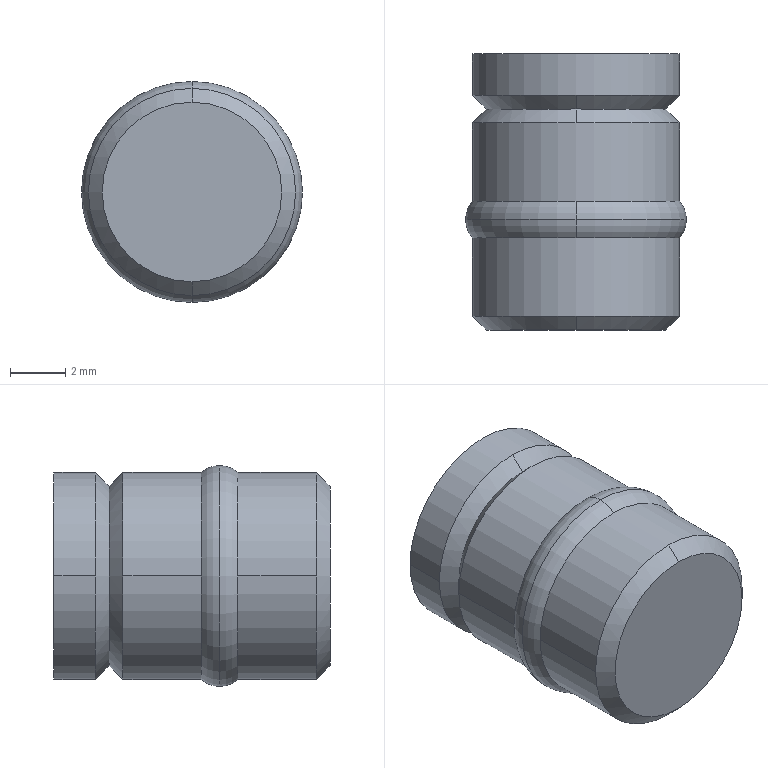Part | Creo | 1 solid | 31 faces | box 8 x 10 x 8 mm | volume 431.828 mm3 | plane 15 | cylinder 6 | cone 6 | torus 4 | commonest cylinder face diameters 7.5 x6
STEP:
#1=CARTESIAN_POINT('',(0.,0.,0.));
#2=DIRECTION('',(0.,0.,1.));
#3=DIRECTION('',(1.,0.,0.));
#4=AXIS2_PLACEMENT_3D('',#1,#2,#3);
#5=CARTESIAN_POINT('',(-58.,4.9,6.673));
#6=VERTEX_POINT('',#5);
#7=CARTESIAN_POINT('',(-59.5,4.9,6.673));
#8=VERTEX_POINT('',#7);
#9=CARTESIAN_POINT('',(-58.,4.9,6.673));
#10=DIRECTION('',(-1.,0.,0.));
#11=VECTOR('',#10,1.5);
#12=LINE('',#9,#11);
#13=EDGE_CURVE('',#6,#8,#12,.T.);
#14=ORIENTED_EDGE('',*,*,#13,.F.);
#15=CARTESIAN_POINT('',(-58.,5.9,6.673));
#16=VERTEX_POINT('',#15);
#17=CARTESIAN_POINT('',(-58.,5.9,6.673));
#18=DIRECTION('',(0.,-1.,0.));
#19=VECTOR('',#18,1.);
#20=LINE('',#17,#19);
#21=EDGE_CURVE('',#16,#6,#20,.T.);
#22=ORIENTED_EDGE('',*,*,#21,.F.);
#23=CARTESIAN_POINT('',(-59.5,5.9,6.673));
#24=VERTEX_POINT('',#23);
#25=CARTESIAN_POINT('',(-58.,5.9,6.673));
#26=DIRECTION('',(-1.,0.,0.));
#27=VECTOR('',#26,1.5);
#28=LINE('',#25,#27);
#29=EDGE_CURVE('',#16,#24,#28,.T.);
#30=ORIENTED_EDGE('',*,*,#29,.T.);
#31=CARTESIAN_POINT('',(-59.5,5.9,6.673));
#32=DIRECTION('',(0.,-1.,0.));
#33=VECTOR('',#32,1.);
#34=LINE('',#31,#33);
#35=EDGE_CURVE('',#24,#8,#34,.T.);
#36=ORIENTED_EDGE('',*,*,#35,.T.);
#37=EDGE_LOOP('',(#14,#22,#30,#36));
#38=FACE_OUTER_BOUND('',#37,.F.);
#39=CARTESIAN_POINT('',(-60.,5.4,6.673));
#40=DIRECTION('',(0.,0.,1.));
#41=DIRECTION('',(0.,1.,0.));
#42=AXIS2_PLACEMENT_3D('',#39,#40,#41);
#43=PLANE('',#42);
#44=ADVANCED_FACE('',(#38),#43,.F.);
#45=CARTESIAN_POINT('',(-59.5,4.9,5.673));
#46=VERTEX_POINT('',#45);
#47=CARTESIAN_POINT('',(-58.,4.9,5.673));
#48=VERTEX_POINT('',#47);
#49=CARTESIAN_POINT('',(-59.5,4.9,5.673));
#50=DIRECTION('',(1.,0.,0.));
#51=VECTOR('',#50,1.5);
#52=LINE('',#49,#51);
#53=EDGE_CURVE('',#46,#48,#52,.T.);
#54=ORIENTED_EDGE('',*,*,#53,.T.);
#55=CARTESIAN_POINT('',(-58.,4.9,5.673));
#56=DIRECTION('',(0.,0.,1.));
#57=VECTOR('',#56,1.);
#58=LINE('',#55,#57);
#59=EDGE_CURVE('',#48,#6,#58,.T.);
#60=ORIENTED_EDGE('',*,*,#59,.T.);
#61=ORIENTED_EDGE('',*,*,#13,.T.);
#62=CARTESIAN_POINT('',(-59.5,4.9,8.172));
#63=VERTEX_POINT('',#62);
#64=CARTESIAN_POINT('',(-59.5,4.9,8.172));
#65=DIRECTION('',(0.,0.,-1.));
#66=VECTOR('',#65,1.5);
#67=LINE('',#64,#66);
#68=EDGE_CURVE('',#63,#8,#67,.T.);
#69=ORIENTED_EDGE('',*,*,#68,.F.);
#70=CARTESIAN_POINT('',(-60.5,4.9,8.172));
#71=VERTEX_POINT('',#70);
#72=CARTESIAN_POINT('',(-60.5,4.9,8.172));
#73=DIRECTION('',(1.,0.,0.));
#74=VECTOR('',#73,1.);
#75=LINE('',#72,#74);
#76=EDGE_CURVE('',#71,#63,#75,.T.);
#77=ORIENTED_EDGE('',*,*,#76,.F.);
#78=CARTESIAN_POINT('',(-60.5,4.9,6.673));
#79=VERTEX_POINT('',#78);
#80=CARTESIAN_POINT('',(-60.5,4.9,8.172));
#81=DIRECTION('',(0.,0.,-1.));
#82=VECTOR('',#81,1.5);
#83=LINE('',#80,#82);
#84=EDGE_CURVE('',#71,#79,#83,.T.);
#85=ORIENTED_EDGE('',*,*,#84,.T.);
#86=CARTESIAN_POINT('',(-62.,4.9,6.673));
#87=VERTEX_POINT('',#86);
#88=CARTESIAN_POINT('',(-60.5,4.9,6.673));
#89=DIRECTION('',(-1.,0.,0.));
#90=VECTOR('',#89,1.5);
#91=LINE('',#88,#90);
#92=EDGE_CURVE('',#79,#87,#91,.T.);
#93=ORIENTED_EDGE('',*,*,#92,.T.);
#94=CARTESIAN_POINT('',(-62.,4.9,5.673));
#95=VERTEX_POINT('',#94);
#96=CARTESIAN_POINT('',(-62.,4.9,5.673));
#97=DIRECTION('',(0.,0.,1.));
#98=VECTOR('',#97,1.);
#99=LINE('',#96,#98);
#100=EDGE_CURVE('',#95,#87,#99,.T.);
#101=ORIENTED_EDGE('',*,*,#100,.F.);
#102=CARTESIAN_POINT('',(-60.5,4.9,5.673));
#103=VERTEX_POINT('',#102);
#104=CARTESIAN_POINT('',(-62.,4.9,5.673));
#105=DIRECTION('',(1.,0.,0.));
#106=VECTOR('',#105,1.5);
#107=LINE('',#104,#106);
#108=EDGE_CURVE('',#95,#103,#107,.T.);
#109=ORIENTED_EDGE('',*,*,#108,.T.);
#110=CARTESIAN_POINT('',(-60.5,4.9,4.173));
#111=VERTEX_POINT('',#110);
#112=CARTESIAN_POINT('',(-60.5,4.9,5.673));
#113=DIRECTION('',(0.,0.,-1.));
#114=VECTOR('',#113,1.5);
#115=LINE('',#112,#114);
#116=EDGE_CURVE('',#103,#111,#115,.T.);
#117=ORIENTED_EDGE('',*,*,#116,.T.);
#118=CARTESIAN_POINT('',(-59.5,4.9,4.173));
#119=VERTEX_POINT('',#118);
#120=CARTESIAN_POINT('',(-59.5,4.9,4.173));
#121=DIRECTION('',(-1.,0.,0.));
#122=VECTOR('',#121,1.);
#123=LINE('',#120,#122);
#124=EDGE_CURVE('',#119,#111,#123,.T.);
#125=ORIENTED_EDGE('',*,*,#124,.F.);
#126=CARTESIAN_POINT('',(-59.5,4.9,5.673));
#127=DIRECTION('',(0.,0.,-1.));
#128=VECTOR('',#127,1.5);
#129=LINE('',#126,#128);
#130=EDGE_CURVE('',#46,#119,#129,.T.);
#131=ORIENTED_EDGE('',*,*,#130,.F.);
#132=EDGE_LOOP('',(#54,#60,#61,#69,#77,#85,#93,#101,#109,#117,#125,#131));
#133=FACE_OUTER_BOUND('',#132,.F.);
#134=CARTESIAN_POINT('',(-60.,4.9,5.673));
#135=DIRECTION('',(0.,-1.,0.));
#136=DIRECTION('',(0.,0.,1.));
#137=AXIS2_PLACEMENT_3D('',#134,#135,#136);
#138=PLANE('',#137);
#139=ADVANCED_FACE('',(#133),#138,.F.);
#140=CARTESIAN_POINT('',(-59.5,5.9,5.673));
#141=VERTEX_POINT('',#140);
#142=CARTESIAN_POINT('',(-58.,5.9,5.673));
#143=VERTEX_POINT('',#142);
#144=CARTESIAN_POINT('',(-59.5,5.9,5.673));
#145=DIRECTION('',(1.,0.,0.));
#146=VECTOR('',#145,1.5);
#147=LINE('',#144,#146);
#148=EDGE_CURVE('',#141,#143,#147,.T.);
#149=ORIENTED_EDGE('',*,*,#148,.T.);
#150=CARTESIAN_POINT('',(-58.,4.9,5.673));
#151=DIRECTION('',(0.,1.,0.));
#152=VECTOR('',#151,1.);
#153=LINE('',#150,#152);
#154=EDGE_CURVE('',#48,#143,#153,.T.);
#155=ORIENTED_EDGE('',*,*,#154,.F.);
#156=ORIENTED_EDGE('',*,*,#53,.F.);
#157=CARTESIAN_POINT('',(-59.5,4.9,5.673));
#158=DIRECTION('',(0.,1.,0.));
#159=VECTOR('',#158,1.);
#160=LINE('',#157,#159);
#161=EDGE_CURVE('',#46,#141,#160,.T.);
#162=ORIENTED_EDGE('',*,*,#161,.T.);
#163=EDGE_LOOP('',(#149,#155,#156,#162));
#164=FACE_OUTER_BOUND('',#163,.F.);
#165=CARTESIAN_POINT('',(-60.,5.4,5.673));
#166=DIRECTION('',(0.,0.,-1.));
#167=DIRECTION('',(0.,-1.,0.));
#168=AXIS2_PLACEMENT_3D('',#165,#166,#167);
#169=PLANE('',#168);
#170=ADVANCED_FACE('',(#164),#169,.F.);
#171=CARTESIAN_POINT('',(-63.75,5.9,6.173));
#172=VERTEX_POINT('',#171);
#173=CARTESIAN_POINT('',(-56.25,5.9,6.173));
#174=VERTEX_POINT('',#173);
#175=CARTESIAN_POINT('',(-60.,5.9,6.173));
#176=DIRECTION('',(0.,1.,0.));
#177=DIRECTION('',(-1.,0.,0.));
#178=AXIS2_PLACEMENT_3D('',#175,#176,#177);
#179=CIRCLE('',#178,3.75);
#180=EDGE_CURVE('',#172,#174,#179,.T.);
#181=ORIENTED_EDGE('',*,*,#180,.F.);
#182=CARTESIAN_POINT('',(-60.,5.9,6.173));
#183=DIRECTION('',(0.,1.,0.));
#184=DIRECTION('',(1.,0.,0.));
#185=AXIS2_PLACEMENT_3D('',#182,#183,#184);
#186=CIRCLE('',#185,3.75);
#187=EDGE_CURVE('',#174,#172,#186,.T.);
#188=ORIENTED_EDGE('',*,*,#187,.F.);
#189=EDGE_LOOP('',(#181,#188));
#190=FACE_OUTER_BOUND('',#189,.F.);
#191=CARTESIAN_POINT('',(-60.5,5.9,5.673));
#192=VERTEX_POINT('',#191);
#193=CARTESIAN_POINT('',(-60.5,5.9,4.173));
#194=VERTEX_POINT('',#193);
#195=CARTESIAN_POINT('',(-60.5,5.9,5.673));
#196=DIRECTION('',(0.,0.,-1.));
#197=VECTOR('',#196,1.5);
#198=LINE('',#195,#197);
#199=EDGE_CURVE('',#192,#194,#198,.T.);
#200=ORIENTED_EDGE('',*,*,#199,.F.);
#201=CARTESIAN_POINT('',(-62.,5.9,5.673));
#202=VERTEX_POINT('',#201);
#203=CARTESIAN_POINT('',(-62.,5.9,5.673));
#204=DIRECTION('',(1.,0.,0.));
#205=VECTOR('',#204,1.5);
#206=LINE('',#203,#205);
#207=EDGE_CURVE('',#202,#192,#206,.T.);
#208=ORIENTED_EDGE('',*,*,#207,.F.);
#209=CARTESIAN_POINT('',(-62.,5.9,6.673));
#210=VERTEX_POINT('',#209);
#211=CARTESIAN_POINT('',(-62.,5.9,6.673));
#212=DIRECTION('',(0.,0.,-1.));
#213=VECTOR('',#212,1.);
#214=LINE('',#211,#213);
#215=EDGE_CURVE('',#210,#202,#214,.T.);
#216=ORIENTED_EDGE('',*,*,#215,.F.);
#217=CARTESIAN_POINT('',(-60.5,5.9,6.673));
#218=VERTEX_POINT('',#217);
#219=CARTESIAN_POINT('',(-60.5,5.9,6.673));
#220=DIRECTION('',(-1.,0.,0.));
#221=VECTOR('',#220,1.5);
#222=LINE('',#219,#221);
#223=EDGE_CURVE('',#218,#210,#222,.T.);
#224=ORIENTED_EDGE('',*,*,#223,.F.);
#225=CARTESIAN_POINT('',(-60.5,5.9,8.172));
#226=VERTEX_POINT('',#225);
#227=CARTESIAN_POINT('',(-60.5,5.9,8.172));
#228=DIRECTION('',(0.,0.,-1.));
#229=VECTOR('',#228,1.5);
#230=LINE('',#227,#229);
#231=EDGE_CURVE('',#226,#218,#230,.T.);
#232=ORIENTED_EDGE('',*,*,#231,.F.);
#233=CARTESIAN_POINT('',(-59.5,5.9,8.172));
#234=VERTEX_POINT('',#233);
#235=CARTESIAN_POINT('',(-59.5,5.9,8.172));
#236=DIRECTION('',(-1.,0.,0.));
#237=VECTOR('',#236,1.);
#238=LINE('',#235,#237);
#239=EDGE_CURVE('',#234,#226,#238,.T.);
#240=ORIENTED_EDGE('',*,*,#239,.F.);
#241=CARTESIAN_POINT('',(-59.5,5.9,8.172));
#242=DIRECTION('',(0.,0.,-1.));
#243=VECTOR('',#242,1.5);
#244=LINE('',#241,#243);
#245=EDGE_CURVE('',#234,#24,#244,.T.);
#246=ORIENTED_EDGE('',*,*,#245,.T.);
#247=ORIENTED_EDGE('',*,*,#29,.F.);
#248=CARTESIAN_POINT('',(-58.,5.9,6.673));
#249=DIRECTION('',(0.,0.,-1.));
#250=VECTOR('',#249,1.);
#251=LINE('',#248,#250);
#252=EDGE_CURVE('',#16,#143,#251,.T.);
#253=ORIENTED_EDGE('',*,*,#252,.T.);
#254=ORIENTED_EDGE('',*,*,#148,.F.);
#255=CARTESIAN_POINT('',(-59.5,5.9,4.173));
#256=VERTEX_POINT('',#255);
#257=CARTESIAN_POINT('',(-59.5,5.9,5.673));
#258=DIRECTION('',(0.,0.,-1.));
#259=VECTOR('',#258,1.5);
#260=LINE('',#257,#259);
#261=EDGE_CURVE('',#141,#256,#260,.T.);
#262=ORIENTED_EDGE('',*,*,#261,.T.);
#263=CARTESIAN_POINT('',(-60.5,5.9,4.173));
#264=DIRECTION('',(1.,0.,0.));
#265=VECTOR('',#264,1.);
#266=LINE('',#263,#265);
#267=EDGE_CURVE('',#194,#256,#266,.T.);
#268=ORIENTED_EDGE('',*,*,#267,.F.);
#269=EDGE_LOOP('',(#200,#208,#216,#224,#232,#240,#246,#247,#253,#254,#262,#268));
#270=FACE_BOUND('',#269,.F.);
#271=CARTESIAN_POINT('',(-60.,5.9,6.173));
#272=DIRECTION('',(0.,1.,0.));
#273=DIRECTION('',(0.,0.,1.));
#274=AXIS2_PLACEMENT_3D('',#271,#272,#273);
#275=PLANE('',#274);
#276=ADVANCED_FACE('',(#190,#270),#275,.T.);
#277=ORIENTED_EDGE('',*,*,#116,.F.);
#278=CARTESIAN_POINT('',(-60.5,5.9,5.673));
#279=DIRECTION('',(0.,-1.,0.));
#280=VECTOR('',#279,1.);
#281=LINE('',#278,#280);
#282=EDGE_CURVE('',#192,#103,#281,.T.);
#283=ORIENTED_EDGE('',*,*,#282,.F.);
#284=ORIENTED_EDGE('',*,*,#199,.T.);
#285=CARTESIAN_POINT('',(-60.5,5.9,4.173));
#286=DIRECTION('',(0.,-1.,0.));
#287=VECTOR('',#286,1.);
#288=LINE('',#285,#287);
#289=EDGE_CURVE('',#194,#111,#288,.T.);
#290=ORIENTED_EDGE('',*,*,#289,.T.);
#291=EDGE_LOOP('',(#277,#283,#284,#290));
#292=FACE_OUTER_BOUND('',#291,.F.);
#293=CARTESIAN_POINT('',(-60.5,5.4,4.173));
#294=DIRECTION('',(-1.,0.,0.));
#295=DIRECTION('',(0.,0.,1.));
#296=AXIS2_PLACEMENT_3D('',#293,#294,#295);
#297=PLANE('',#296);
#298=ADVANCED_FACE('',(#292),#297,.F.);
#299=ORIENTED_EDGE('',*,*,#108,.F.);
#300=CARTESIAN_POINT('',(-62.,5.9,5.673));
#301=DIRECTION('',(0.,-1.,0.));
#302=VECTOR('',#301,1.);
#303=LINE('',#300,#302);
#304=EDGE_CURVE('',#202,#95,#303,.T.);
#305=ORIENTED_EDGE('',*,*,#304,.F.);
#306=ORIENTED_EDGE('',*,*,#207,.T.);
#307=ORIENTED_EDGE('',*,*,#282,.T.);
#308=EDGE_LOOP('',(#299,#305,#306,#307));
#309=FACE_OUTER_BOUND('',#308,.F.);
#310=CARTESIAN_POINT('',(-60.,5.4,5.673));
#311=DIRECTION('',(0.,0.,-1.));
#312=DIRECTION('',(0.,-1.,0.));
#313=AXIS2_PLACEMENT_3D('',#310,#311,#312);
#314=PLANE('',#313);
#315=ADVANCED_FACE('',(#309),#314,.F.);
#316=ORIENTED_EDGE('',*,*,#100,.T.);
#317=CARTESIAN_POINT('',(-62.,4.9,6.673));
#318=DIRECTION('',(0.,1.,0.));
#319=VECTOR('',#318,1.);
#320=LINE('',#317,#319);
#321=EDGE_CURVE('',#87,#210,#320,.T.);
#322=ORIENTED_EDGE('',*,*,#321,.T.);
#323=ORIENTED_EDGE('',*,*,#215,.T.);
#324=ORIENTED_EDGE('',*,*,#304,.T.);
#325=EDGE_LOOP('',(#316,#322,#323,#324));
#326=FACE_OUTER_BOUND('',#325,.F.);
#327=CARTESIAN_POINT('',(-62.,5.4,5.673));
#328=DIRECTION('',(-1.,0.,0.));
#329=DIRECTION('',(0.,0.,1.));
#330=AXIS2_PLACEMENT_3D('',#327,#328,#329);
#331=PLANE('',#330);
#332=ADVANCED_FACE('',(#326),#331,.F.);
#333=ORIENTED_EDGE('',*,*,#223,.T.);
#334=ORIENTED_EDGE('',*,*,#321,.F.);
#335=ORIENTED_EDGE('',*,*,#92,.F.);
#336=CARTESIAN_POINT('',(-60.5,4.9,6.673));
#337=DIRECTION('',(0.,1.,0.));
#338=VECTOR('',#337,1.);
#339=LINE('',#336,#338);
#340=EDGE_CURVE('',#79,#218,#339,.T.);
#341=ORIENTED_EDGE('',*,*,#340,.T.);
#342=EDGE_LOOP('',(#333,#334,#335,#341));
#343=FACE_OUTER_BOUND('',#342,.F.);
#344=CARTESIAN_POINT('',(-60.,5.4,6.673));
#345=DIRECTION('',(0.,0.,1.));
#346=DIRECTION('',(0.,1.,0.));
#347=AXIS2_PLACEMENT_3D('',#344,#345,#346);
#348=PLANE('',#347);
#349=ADVANCED_FACE('',(#343),#348,.F.);
#350=ORIENTED_EDGE('',*,*,#231,.T.);
#351=ORIENTED_EDGE('',*,*,#340,.F.);
#352=ORIENTED_EDGE('',*,*,#84,.F.);
#353=CARTESIAN_POINT('',(-60.5,4.9,8.172));
#354=DIRECTION('',(0.,1.,0.));
#355=VECTOR('',#354,1.);
#356=LINE('',#353,#355);
#357=EDGE_CURVE('',#71,#226,#356,.T.);
#358=ORIENTED_EDGE('',*,*,#357,.T.);
#359=EDGE_LOOP('',(#350,#351,#352,#358));
#360=FACE_OUTER_BOUND('',#359,.F.);
#361=CARTESIAN_POINT('',(-60.5,5.4,4.173));
#362=DIRECTION('',(-1.,0.,0.));
#363=DIRECTION('',(0.,0.,1.));
#364=AXIS2_PLACEMENT_3D('',#361,#362,#363);
#365=PLANE('',#364);
#366=ADVANCED_FACE('',(#360),#365,.F.);
#367=CARTESIAN_POINT('',(-59.5,5.9,8.172));
#368=DIRECTION('',(0.,-1.,0.));
#369=VECTOR('',#368,1.);
#370=LINE('',#367,#369);
#371=EDGE_CURVE('',#234,#63,#370,.T.);
#372=ORIENTED_EDGE('',*,*,#371,.F.);
#373=ORIENTED_EDGE('',*,*,#239,.T.);
#374=ORIENTED_EDGE('',*,*,#357,.F.);
#375=ORIENTED_EDGE('',*,*,#76,.T.);
#376=EDGE_LOOP('',(#372,#373,#374,#375));
#377=FACE_OUTER_BOUND('',#376,.F.);
#378=CARTESIAN_POINT('',(-60.,5.4,8.172));
#379=DIRECTION('',(0.,0.,1.));
#380=DIRECTION('',(0.,1.,0.));
#381=AXIS2_PLACEMENT_3D('',#378,#379,#380);
#382=PLANE('',#381);
#383=ADVANCED_FACE('',(#377),#382,.F.);
#384=ORIENTED_EDGE('',*,*,#68,.T.);
#385=ORIENTED_EDGE('',*,*,#35,.F.);
#386=ORIENTED_EDGE('',*,*,#245,.F.);
#387=ORIENTED_EDGE('',*,*,#371,.T.);
#388=EDGE_LOOP('',(#384,#385,#386,#387));
#389=FACE_OUTER_BOUND('',#388,.F.);
#390=CARTESIAN_POINT('',(-59.5,5.4,4.173));
#391=DIRECTION('',(1.,0.,0.));
#392=DIRECTION('',(0.,0.,-1.));
#393=AXIS2_PLACEMENT_3D('',#390,#391,#392);
#394=PLANE('',#393);
#395=ADVANCED_FACE('',(#389),#394,.F.);
#396=ORIENTED_EDGE('',*,*,#267,.T.);
#397=CARTESIAN_POINT('',(-59.5,4.9,4.173));
#398=DIRECTION('',(0.,1.,0.));
#399=VECTOR('',#398,1.);
#400=LINE('',#397,#399);
#401=EDGE_CURVE('',#119,#256,#400,.T.);
#402=ORIENTED_EDGE('',*,*,#401,.F.);
#403=ORIENTED_EDGE('',*,*,#124,.T.);
#404=ORIENTED_EDGE('',*,*,#289,.F.);
#405=EDGE_LOOP('',(#396,#402,#403,#404));
#406=FACE_OUTER_BOUND('',#405,.F.);
#407=CARTESIAN_POINT('',(-60.,5.4,4.173));
#408=DIRECTION('',(0.,0.,-1.));
#409=DIRECTION('',(0.,-1.,0.));
#410=AXIS2_PLACEMENT_3D('',#407,#408,#409);
#411=PLANE('',#410);
#412=ADVANCED_FACE('',(#406),#411,.F.);
#413=ORIENTED_EDGE('',*,*,#261,.F.);
#414=ORIENTED_EDGE('',*,*,#161,.F.);
#415=ORIENTED_EDGE('',*,*,#130,.T.);
#416=ORIENTED_EDGE('',*,*,#401,.T.);
#417=EDGE_LOOP('',(#413,#414,#415,#416));
#418=FACE_OUTER_BOUND('',#417,.F.);
#419=CARTESIAN_POINT('',(-59.5,5.4,4.173));
#420=DIRECTION('',(1.,0.,0.));
#421=DIRECTION('',(0.,0.,-1.));
#422=AXIS2_PLACEMENT_3D('',#419,#420,#421);
#423=PLANE('',#422);
#424=ADVANCED_FACE('',(#418),#423,.F.);
#425=ORIENTED_EDGE('',*,*,#252,.F.);
#426=ORIENTED_EDGE('',*,*,#21,.T.);
#427=ORIENTED_EDGE('',*,*,#59,.F.);
#428=ORIENTED_EDGE('',*,*,#154,.T.);
#429=EDGE_LOOP('',(#425,#426,#427,#428));
#430=FACE_OUTER_BOUND('',#429,.F.);
#431=CARTESIAN_POINT('',(-58.,5.4,5.673));
#432=DIRECTION('',(1.,0.,0.));
#433=DIRECTION('',(0.,0.,-1.));
#434=AXIS2_PLACEMENT_3D('',#431,#432,#433);
#435=PLANE('',#434);
#436=ADVANCED_FACE('',(#430),#435,.F.);
#437=CARTESIAN_POINT('',(-60.,4.4,9.922));
#438=VERTEX_POINT('',#437);
#439=CARTESIAN_POINT('',(-63.75,4.4,6.173));
#440=VERTEX_POINT('',#439);
#441=CARTESIAN_POINT('',(-60.,4.4,6.173));
#442=DIRECTION('',(0.,-1.,0.));
#443=DIRECTION('',(0.,0.,1.));
#444=AXIS2_PLACEMENT_3D('',#441,#442,#443);
#445=CIRCLE('',#444,3.75);
#446=EDGE_CURVE('',#438,#440,#445,.T.);
#447=ORIENTED_EDGE('',*,*,#446,.T.);
#448=CARTESIAN_POINT('',(-63.75,5.9,6.173));
#449=DIRECTION('',(0.,-1.,0.));
#450=VECTOR('',#449,1.5);
#451=LINE('',#448,#450);
#452=EDGE_CURVE('',#172,#440,#451,.T.);
#453=ORIENTED_EDGE('',*,*,#452,.F.);
#454=ORIENTED_EDGE('',*,*,#180,.T.);
#455=CARTESIAN_POINT('',(-56.25,4.4,6.173));
#456=VERTEX_POINT('',#455);
#457=CARTESIAN_POINT('',(-56.25,5.9,6.173));
#458=DIRECTION('',(0.,-1.,0.));
#459=VECTOR('',#458,1.5);
#460=LINE('',#457,#459);
#461=EDGE_CURVE('',#174,#456,#460,.T.);
#462=ORIENTED_EDGE('',*,*,#461,.T.);
#463=CARTESIAN_POINT('',(-60.,4.4,6.173));
#464=DIRECTION('',(0.,-1.,0.));
#465=DIRECTION('',(1.,0.,0.));
#466=AXIS2_PLACEMENT_3D('',#463,#464,#465);
#467=CIRCLE('',#466,3.75);
#468=EDGE_CURVE('',#456,#438,#467,.T.);
#469=ORIENTED_EDGE('',*,*,#468,.T.);
#470=EDGE_LOOP('',(#447,#453,#454,#462,#469));
#471=FACE_OUTER_BOUND('',#470,.F.);
#472=CARTESIAN_POINT('',(-60.,5.9,6.173));
#473=DIRECTION('',(0.,-1.,0.));
#474=DIRECTION('',(-1.,0.,0.));
#475=AXIS2_PLACEMENT_3D('',#472,#473,#474);
#476=CYLINDRICAL_SURFACE('',#475,3.75);
#477=ADVANCED_FACE('',(#471),#476,.T.);
#478=CARTESIAN_POINT('',(-60.,3.9,2.922));
#479=VERTEX_POINT('',#478);
#480=CARTESIAN_POINT('',(-60.,3.9,9.422));
#481=VERTEX_POINT('',#480);
#482=CARTESIAN_POINT('',(-60.,3.9,6.173));
#483=DIRECTION('',(0.,1.,0.));
#484=DIRECTION('',(0.,0.,-1.));
#485=AXIS2_PLACEMENT_3D('',#482,#483,#484);
#486=CIRCLE('',#485,3.25);
#487=EDGE_CURVE('',#479,#481,#486,.T.);
#488=ORIENTED_EDGE('',*,*,#487,.F.);
#489=CARTESIAN_POINT('',(-60.,4.4,2.422));
#490=VERTEX_POINT('',#489);
#491=CARTESIAN_POINT('',(-60.,3.9,2.922));
#492=DIRECTION('',(0.,0.7071,-0.7071));
#493=VECTOR('',#492,0.7071);
#494=LINE('',#491,#493);
#495=EDGE_CURVE('',#479,#490,#494,.T.);
#496=ORIENTED_EDGE('',*,*,#495,.T.);
#497=CARTESIAN_POINT('',(-60.,4.4,6.173));
#498=DIRECTION('',(0.,-1.,0.));
#499=DIRECTION('',(-1.,0.,0.));
#500=AXIS2_PLACEMENT_3D('',#497,#498,#499);
#501=CIRCLE('',#500,3.75);
#502=EDGE_CURVE('',#440,#490,#501,.T.);
#503=ORIENTED_EDGE('',*,*,#502,.F.);
#504=ORIENTED_EDGE('',*,*,#446,.F.);
#505=CARTESIAN_POINT('',(-60.,3.9,9.422));
#506=DIRECTION('',(0.,0.7071,0.7071));
#507=VECTOR('',#506,0.7071);
#508=LINE('',#505,#507);
#509=EDGE_CURVE('',#481,#438,#508,.T.);
#510=ORIENTED_EDGE('',*,*,#509,.F.);
#511=EDGE_LOOP('',(#488,#496,#503,#504,#510));
#512=FACE_OUTER_BOUND('',#511,.F.);
#513=CARTESIAN_POINT('',(-60.,4.15,6.173));
#514=DIRECTION('',(0.,1.,0.));
#515=DIRECTION('',(0.,0.,1.));
#516=AXIS2_PLACEMENT_3D('',#513,#514,#515);
#517=CONICAL_SURFACE('',#516,3.5,45.);
#518=ADVANCED_FACE('',(#512),#517,.T.);
#519=ORIENTED_EDGE('',*,*,#487,.T.);
#520=CARTESIAN_POINT('',(-60.,3.4,9.922));
#521=VERTEX_POINT('',#520);
#522=CARTESIAN_POINT('',(-60.,3.9,9.422));
#523=DIRECTION('',(0.,-0.7071,0.7071));
#524=VECTOR('',#523,0.7071);
#525=LINE('',#522,#524);
#526=EDGE_CURVE('',#481,#521,#525,.T.);
#527=ORIENTED_EDGE('',*,*,#526,.T.);
#528=CARTESIAN_POINT('',(-63.75,3.4,6.173));
#529=VERTEX_POINT('',#528);
#530=CARTESIAN_POINT('',(-60.,3.4,6.173));
#531=DIRECTION('',(0.,1.,0.));
#532=DIRECTION('',(-1.,0.,0.));
#533=AXIS2_PLACEMENT_3D('',#530,#531,#532);
#534=CIRCLE('',#533,3.75);
#535=EDGE_CURVE('',#529,#521,#534,.T.);
#536=ORIENTED_EDGE('',*,*,#535,.F.);
#537=CARTESIAN_POINT('',(-60.,3.4,2.422));
#538=VERTEX_POINT('',#537);
#539=CARTESIAN_POINT('',(-60.,3.4,6.173));
#540=DIRECTION('',(0.,1.,0.));
#541=DIRECTION('',(0.,0.,-1.));
#542=AXIS2_PLACEMENT_3D('',#539,#540,#541);
#543=CIRCLE('',#542,3.75);
#544=EDGE_CURVE('',#538,#529,#543,.T.);
#545=ORIENTED_EDGE('',*,*,#544,.F.);
#546=CARTESIAN_POINT('',(-60.,3.9,2.922));
#547=DIRECTION('',(0.,-0.7071,-0.7071));
#548=VECTOR('',#547,0.7071);
#549=LINE('',#546,#548);
#550=EDGE_CURVE('',#479,#538,#549,.T.);
#551=ORIENTED_EDGE('',*,*,#550,.F.);
#552=EDGE_LOOP('',(#519,#527,#536,#545,#551));
#553=FACE_OUTER_BOUND('',#552,.F.);
#554=CARTESIAN_POINT('',(-60.,3.65,6.173));
#555=DIRECTION('',(0.,-1.,0.));
#556=DIRECTION('',(0.,0.,-1.));
#557=AXIS2_PLACEMENT_3D('',#554,#555,#556);
#558=CONICAL_SURFACE('',#557,3.5,45.);
#559=ADVANCED_FACE('',(#553),#558,.T.);
#560=CARTESIAN_POINT('',(-60.,3.9,6.173));
#561=DIRECTION('',(0.,1.,0.));
#562=DIRECTION('',(0.,0.,1.));
#563=AXIS2_PLACEMENT_3D('',#560,#561,#562);
#564=CIRCLE('',#563,3.25);
#565=EDGE_CURVE('',#481,#479,#564,.T.);
#566=ORIENTED_EDGE('',*,*,#565,.T.);
#567=ORIENTED_EDGE('',*,*,#550,.T.);
#568=CARTESIAN_POINT('',(-56.25,3.4,6.173));
#569=VERTEX_POINT('',#568);
#570=CARTESIAN_POINT('',(-60.,3.4,6.173));
#571=DIRECTION('',(0.,1.,0.));
#572=DIRECTION('',(1.,0.,0.));
#573=AXIS2_PLACEMENT_3D('',#570,#571,#572);
#574=CIRCLE('',#573,3.75);
#575=EDGE_CURVE('',#569,#538,#574,.T.);
#576=ORIENTED_EDGE('',*,*,#575,.F.);
#577=CARTESIAN_POINT('',(-60.,3.4,6.173));
#578=DIRECTION('',(0.,1.,0.));
#579=DIRECTION('',(0.,0.,1.));
#580=AXIS2_PLACEMENT_3D('',#577,#578,#579);
#581=CIRCLE('',#580,3.75);
#582=EDGE_CURVE('',#521,#569,#581,.T.);
#583=ORIENTED_EDGE('',*,*,#582,.F.);
#584=ORIENTED_EDGE('',*,*,#526,.F.);
#585=EDGE_LOOP('',(#566,#567,#576,#583,#584));
#586=FACE_OUTER_BOUND('',#585,.F.);
#587=CARTESIAN_POINT('',(-60.,3.65,6.173));
#588=DIRECTION('',(0.,-1.,0.));
#589=DIRECTION('',(0.,0.,-1.));
#590=AXIS2_PLACEMENT_3D('',#587,#588,#589);
#591=CONICAL_SURFACE('',#590,3.5,45.);
#592=ADVANCED_FACE('',(#586),#591,.T.);
#593=ORIENTED_EDGE('',*,*,#565,.F.);
#594=ORIENTED_EDGE('',*,*,#509,.T.);
#595=ORIENTED_EDGE('',*,*,#468,.F.);
#596=CARTESIAN_POINT('',(-60.,4.4,6.173));
#597=DIRECTION('',(0.,-1.,0.));
#598=DIRECTION('',(0.,0.,-1.));
#599=AXIS2_PLACEMENT_3D('',#596,#597,#598);
#600=CIRCLE('',#599,3.75);
#601=EDGE_CURVE('',#490,#456,#600,.T.);
#602=ORIENTED_EDGE('',*,*,#601,.F.);
#603=ORIENTED_EDGE('',*,*,#495,.F.);
#604=EDGE_LOOP('',(#593,#594,#595,#602,#603));
#605=FACE_OUTER_BOUND('',#604,.F.);
#606=CARTESIAN_POINT('',(-60.,4.15,6.173));
#607=DIRECTION('',(0.,1.,0.));
#608=DIRECTION('',(0.,0.,1.));
#609=AXIS2_PLACEMENT_3D('',#606,#607,#608);
#610=CONICAL_SURFACE('',#609,3.5,45.);
#611=ADVANCED_FACE('',(#605),#610,.T.);
#612=ORIENTED_EDGE('',*,*,#502,.T.);
#613=ORIENTED_EDGE('',*,*,#601,.T.);
#614=ORIENTED_EDGE('',*,*,#461,.F.);
#615=ORIENTED_EDGE('',*,*,#187,.T.);
#616=ORIENTED_EDGE('',*,*,#452,.T.);
#617=EDGE_LOOP('',(#612,#613,#614,#615,#616));
#618=FACE_OUTER_BOUND('',#617,.F.);
#619=CARTESIAN_POINT('',(-60.,5.9,6.173));
#620=DIRECTION('',(0.,-1.,0.));
#621=DIRECTION('',(-1.,0.,0.));
#622=AXIS2_PLACEMENT_3D('',#619,#620,#621);
#623=CYLINDRICAL_SURFACE('',#622,3.75);
#624=ADVANCED_FACE('',(#618),#623,.T.);
#625=CARTESIAN_POINT('',(-63.75,0.5614,6.173));
#626=VERTEX_POINT('',#625);
#627=CARTESIAN_POINT('',(-60.,0.5614,2.422));
#628=VERTEX_POINT('',#627);
#629=CARTESIAN_POINT('',(-60.,0.5614,6.173));
#630=DIRECTION('',(0.,-1.,0.));
#631=DIRECTION('',(-1.,0.,0.));
#632=AXIS2_PLACEMENT_3D('',#629,#630,#631);
#633=CIRCLE('',#632,3.75);
#634=EDGE_CURVE('',#626,#628,#633,.T.);
#635=ORIENTED_EDGE('',*,*,#634,.T.);
#636=CARTESIAN_POINT('',(-56.25,0.5614,6.173));
#637=VERTEX_POINT('',#636);
#638=CARTESIAN_POINT('',(-60.,0.5614,6.173));
#639=DIRECTION('',(0.,-1.,0.));
#640=DIRECTION('',(0.,0.,-1.));
#641=AXIS2_PLACEMENT_3D('',#638,#639,#640);
#642=CIRCLE('',#641,3.75);
#643=EDGE_CURVE('',#628,#637,#642,.T.);
#644=ORIENTED_EDGE('',*,*,#643,.T.);
#645=CARTESIAN_POINT('',(-56.25,3.4,6.173));
#646=DIRECTION('',(0.,-1.,0.));
#647=VECTOR('',#646,2.839);
#648=LINE('',#645,#647);
#649=EDGE_CURVE('',#569,#637,#648,.T.);
#650=ORIENTED_EDGE('',*,*,#649,.F.);
#651=ORIENTED_EDGE('',*,*,#575,.T.);
#652=ORIENTED_EDGE('',*,*,#544,.T.);
#653=CARTESIAN_POINT('',(-63.75,3.4,6.173));
#654=DIRECTION('',(0.,-1.,0.));
#655=VECTOR('',#654,2.839);
#656=LINE('',#653,#655);
#657=EDGE_CURVE('',#529,#626,#656,.T.);
#658=ORIENTED_EDGE('',*,*,#657,.T.);
#659=EDGE_LOOP('',(#635,#644,#650,#651,#652,#658));
#660=FACE_OUTER_BOUND('',#659,.F.);
#661=CARTESIAN_POINT('',(-60.,3.9,6.173));
#662=DIRECTION('',(0.,-1.,0.));
#663=DIRECTION('',(-1.,0.,0.));
#664=AXIS2_PLACEMENT_3D('',#661,#662,#663);
#665=CYLINDRICAL_SURFACE('',#664,3.75);
#666=ADVANCED_FACE('',(#660),#665,.T.);
#667=CARTESIAN_POINT('',(-60.,0.5614,9.922));
#668=VERTEX_POINT('',#667);
#669=CARTESIAN_POINT('',(-60.,0.5614,6.173));
#670=DIRECTION('',(0.,-1.,0.));
#671=DIRECTION('',(0.,0.,1.));
#672=AXIS2_PLACEMENT_3D('',#669,#670,#671);
#673=CIRCLE('',#672,3.75);
#674=EDGE_CURVE('',#668,#626,#673,.T.);
#675=ORIENTED_EDGE('',*,*,#674,.F.);
#676=CARTESIAN_POINT('',(-60.,-0.1,10.172));
#677=VERTEX_POINT('',#676);
#678=CARTESIAN_POINT('',(-60.,-0.1,9.172));
#679=DIRECTION('',(-1.,0.,0.));
#680=DIRECTION('',(0.,0.,1.));
#681=AXIS2_PLACEMENT_3D('',#678,#679,#680);
#682=CIRCLE('',#681,1.);
#683=EDGE_CURVE('',#677,#668,#682,.T.);
#684=ORIENTED_EDGE('',*,*,#683,.F.);
#685=CARTESIAN_POINT('',(-60.,-0.1,2.172));
#686=VERTEX_POINT('',#685);
#687=CARTESIAN_POINT('',(-60.,-0.1,6.173));
#688=DIRECTION('',(0.,1.,0.));
#689=DIRECTION('',(0.,0.,-1.));
#690=AXIS2_PLACEMENT_3D('',#687,#688,#689);
#691=CIRCLE('',#690,4.);
#692=EDGE_CURVE('',#686,#677,#691,.T.);
#693=ORIENTED_EDGE('',*,*,#692,.F.);
#694=CARTESIAN_POINT('',(-60.,-0.1,3.172));
#695=DIRECTION('',(1.,0.,0.));
#696=DIRECTION('',(0.,0.,-1.));
#697=AXIS2_PLACEMENT_3D('',#694,#695,#696);
#698=CIRCLE('',#697,1.);
#699=EDGE_CURVE('',#686,#628,#698,.T.);
#700=ORIENTED_EDGE('',*,*,#699,.T.);
#701=ORIENTED_EDGE('',*,*,#634,.F.);
#702=EDGE_LOOP('',(#675,#684,#693,#700,#701));
#703=FACE_OUTER_BOUND('',#702,.F.);
#704=CARTESIAN_POINT('',(-60.,-0.1,6.173));
#705=DIRECTION('',(0.,1.,0.));
#706=DIRECTION('',(0.,0.,1.));
#707=AXIS2_PLACEMENT_3D('',#704,#705,#706);
#708=TOROIDAL_SURFACE('',#707,3.,1.);
#709=ADVANCED_FACE('',(#703),#708,.T.);
#710=ORIENTED_EDGE('',*,*,#674,.T.);
#711=ORIENTED_EDGE('',*,*,#657,.F.);
#712=ORIENTED_EDGE('',*,*,#535,.T.);
#713=ORIENTED_EDGE('',*,*,#582,.T.);
#714=ORIENTED_EDGE('',*,*,#649,.T.);
#715=CARTESIAN_POINT('',(-60.,0.5614,6.173));
#716=DIRECTION('',(0.,-1.,0.));
#717=DIRECTION('',(1.,0.,0.));
#718=AXIS2_PLACEMENT_3D('',#715,#716,#717);
#719=CIRCLE('',#718,3.75);
#720=EDGE_CURVE('',#637,#668,#719,.T.);
#721=ORIENTED_EDGE('',*,*,#720,.T.);
#722=EDGE_LOOP('',(#710,#711,#712,#713,#714,#721));
#723=FACE_OUTER_BOUND('',#722,.F.);
#724=CARTESIAN_POINT('',(-60.,3.9,6.173));
#725=DIRECTION('',(0.,-1.,0.));
#726=DIRECTION('',(-1.,0.,0.));
#727=AXIS2_PLACEMENT_3D('',#724,#725,#726);
#728=CYLINDRICAL_SURFACE('',#727,3.75);
#729=ADVANCED_FACE('',(#723),#728,.T.);
#730=ORIENTED_EDGE('',*,*,#643,.F.);
#731=ORIENTED_EDGE('',*,*,#699,.F.);
#732=CARTESIAN_POINT('',(-60.,-0.1,6.173));
#733=DIRECTION('',(0.,1.,0.));
#734=DIRECTION('',(0.,0.,1.));
#735=AXIS2_PLACEMENT_3D('',#732,#733,#734);
#736=CIRCLE('',#735,4.);
#737=EDGE_CURVE('',#677,#686,#736,.T.);
#738=ORIENTED_EDGE('',*,*,#737,.F.);
#739=ORIENTED_EDGE('',*,*,#683,.T.);
#740=ORIENTED_EDGE('',*,*,#720,.F.);
#741=EDGE_LOOP('',(#730,#731,#738,#739,#740));
#742=FACE_OUTER_BOUND('',#741,.F.);
#743=CARTESIAN_POINT('',(-60.,-0.1,6.173));
#744=DIRECTION('',(0.,1.,0.));
#745=DIRECTION('',(0.,0.,1.));
#746=AXIS2_PLACEMENT_3D('',#743,#744,#745);
#747=TOROIDAL_SURFACE('',#746,3.,1.);
#748=ADVANCED_FACE('',(#742),#747,.T.);
#749=CARTESIAN_POINT('',(-60.,-0.7614,9.922));
#750=VERTEX_POINT('',#749);
#751=CARTESIAN_POINT('',(-56.25,-0.7614,6.173));
#752=VERTEX_POINT('',#751);
#753=CARTESIAN_POINT('',(-60.,-0.7614,6.173));
#754=DIRECTION('',(0.,1.,0.));
#755=DIRECTION('',(0.,0.,1.));
#756=AXIS2_PLACEMENT_3D('',#753,#754,#755);
#757=CIRCLE('',#756,3.75);
#758=EDGE_CURVE('',#750,#752,#757,.T.);
#759=ORIENTED_EDGE('',*,*,#758,.F.);
#760=CARTESIAN_POINT('',(-60.,-0.1,9.172));
#761=DIRECTION('',(-1.,0.,0.));
#762=DIRECTION('',(0.,-0.6614,0.75));
#763=AXIS2_PLACEMENT_3D('',#760,#761,#762);
#764=CIRCLE('',#763,1.);
#765=EDGE_CURVE('',#750,#677,#764,.T.);
#766=ORIENTED_EDGE('',*,*,#765,.T.);
#767=ORIENTED_EDGE('',*,*,#737,.T.);
#768=CARTESIAN_POINT('',(-60.,-0.7614,2.422));
#769=VERTEX_POINT('',#768);
#770=CARTESIAN_POINT('',(-60.,-0.1,3.172));
#771=DIRECTION('',(1.,0.,0.));
#772=DIRECTION('',(0.,-0.6614,-0.75));
#773=AXIS2_PLACEMENT_3D('',#770,#771,#772);
#774=CIRCLE('',#773,1.);
#775=EDGE_CURVE('',#769,#686,#774,.T.);
#776=ORIENTED_EDGE('',*,*,#775,.F.);
#777=CARTESIAN_POINT('',(-60.,-0.7614,6.173));
#778=DIRECTION('',(0.,1.,0.));
#779=DIRECTION('',(1.,0.,0.));
#780=AXIS2_PLACEMENT_3D('',#777,#778,#779);
#781=CIRCLE('',#780,3.75);
#782=EDGE_CURVE('',#752,#769,#781,.T.);
#783=ORIENTED_EDGE('',*,*,#782,.F.);
#784=EDGE_LOOP('',(#759,#766,#767,#776,#783));
#785=FACE_OUTER_BOUND('',#784,.F.);
#786=CARTESIAN_POINT('',(-60.,-0.1,6.173));
#787=DIRECTION('',(0.,1.,0.));
#788=DIRECTION('',(0.,0.,1.));
#789=AXIS2_PLACEMENT_3D('',#786,#787,#788);
#790=TOROIDAL_SURFACE('',#789,3.,1.);
#791=ADVANCED_FACE('',(#785),#790,.T.);
#792=CARTESIAN_POINT('',(-63.75,-0.7614,6.173));
#793=VERTEX_POINT('',#792);
#794=CARTESIAN_POINT('',(-60.,-0.7614,6.173));
#795=DIRECTION('',(0.,1.,0.));
#796=DIRECTION('',(-1.,0.,0.));
#797=AXIS2_PLACEMENT_3D('',#794,#795,#796);
#798=CIRCLE('',#797,3.75);
#799=EDGE_CURVE('',#793,#750,#798,.T.);
#800=ORIENTED_EDGE('',*,*,#799,.T.);
#801=ORIENTED_EDGE('',*,*,#758,.T.);
#802=CARTESIAN_POINT('',(-56.25,-3.6,6.173));
#803=VERTEX_POINT('',#802);
#804=CARTESIAN_POINT('',(-56.25,-0.7614,6.173));
#805=DIRECTION('',(0.,-1.,0.));
#806=VECTOR('',#805,2.839);
#807=LINE('',#804,#806);
#808=EDGE_CURVE('',#752,#803,#807,.T.);
#809=ORIENTED_EDGE('',*,*,#808,.T.);
#810=CARTESIAN_POINT('',(-60.,-3.6,9.922));
#811=VERTEX_POINT('',#810);
#812=CARTESIAN_POINT('',(-60.,-3.6,6.173));
#813=DIRECTION('',(0.,-1.,0.));
#814=DIRECTION('',(1.,0.,0.));
#815=AXIS2_PLACEMENT_3D('',#812,#813,#814);
#816=CIRCLE('',#815,3.75);
#817=EDGE_CURVE('',#803,#811,#816,.T.);
#818=ORIENTED_EDGE('',*,*,#817,.T.);
#819=CARTESIAN_POINT('',(-63.75,-3.6,6.173));
#820=VERTEX_POINT('',#819);
#821=CARTESIAN_POINT('',(-60.,-3.6,6.173));
#822=DIRECTION('',(0.,-1.,0.));
#823=DIRECTION('',(0.,0.,1.));
#824=AXIS2_PLACEMENT_3D('',#821,#822,#823);
#825=CIRCLE('',#824,3.75);
#826=EDGE_CURVE('',#811,#820,#825,.T.);
#827=ORIENTED_EDGE('',*,*,#826,.T.);
#828=CARTESIAN_POINT('',(-63.75,-0.7614,6.173));
#829=DIRECTION('',(0.,-1.,0.));
#830=VECTOR('',#829,2.839);
#831=LINE('',#828,#830);
#832=EDGE_CURVE('',#793,#820,#831,.T.);
#833=ORIENTED_EDGE('',*,*,#832,.F.);
#834=EDGE_LOOP('',(#800,#801,#809,#818,#827,#833));
#835=FACE_OUTER_BOUND('',#834,.F.);
#836=CARTESIAN_POINT('',(-60.,3.9,6.173));
#837=DIRECTION('',(0.,-1.,0.));
#838=DIRECTION('',(-1.,0.,0.));
#839=AXIS2_PLACEMENT_3D('',#836,#837,#838);
#840=CYLINDRICAL_SURFACE('',#839,3.75);
#841=ADVANCED_FACE('',(#835),#840,.T.);
#842=CARTESIAN_POINT('',(-60.,-0.7614,6.173));
#843=DIRECTION('',(0.,1.,0.));
#844=DIRECTION('',(0.,0.,-1.));
#845=AXIS2_PLACEMENT_3D('',#842,#843,#844);
#846=CIRCLE('',#845,3.75);
#847=EDGE_CURVE('',#769,#793,#846,.T.);
#848=ORIENTED_EDGE('',*,*,#847,.F.);
#849=ORIENTED_EDGE('',*,*,#775,.T.);
#850=ORIENTED_EDGE('',*,*,#692,.T.);
#851=ORIENTED_EDGE('',*,*,#765,.F.);
#852=ORIENTED_EDGE('',*,*,#799,.F.);
#853=EDGE_LOOP('',(#848,#849,#850,#851,#852));
#854=FACE_OUTER_BOUND('',#853,.F.);
#855=CARTESIAN_POINT('',(-60.,-0.1,6.173));
#856=DIRECTION('',(0.,1.,0.));
#857=DIRECTION('',(0.,0.,1.));
#858=AXIS2_PLACEMENT_3D('',#855,#856,#857);
#859=TOROIDAL_SURFACE('',#858,3.,1.);
#860=ADVANCED_FACE('',(#854),#859,.T.);
#861=ORIENTED_EDGE('',*,*,#847,.T.);
#862=ORIENTED_EDGE('',*,*,#832,.T.);
#863=CARTESIAN_POINT('',(-60.,-3.6,2.422));
#864=VERTEX_POINT('',#863);
#865=CARTESIAN_POINT('',(-60.,-3.6,6.173));
#866=DIRECTION('',(0.,-1.,0.));
#867=DIRECTION('',(-1.,0.,0.));
#868=AXIS2_PLACEMENT_3D('',#865,#866,#867);
#869=CIRCLE('',#868,3.75);
#870=EDGE_CURVE('',#820,#864,#869,.T.);
#871=ORIENTED_EDGE('',*,*,#870,.T.);
#872=CARTESIAN_POINT('',(-60.,-3.6,6.173));
#873=DIRECTION('',(0.,-1.,0.));
#874=DIRECTION('',(0.,0.,-1.));
#875=AXIS2_PLACEMENT_3D('',#872,#873,#874);
#876=CIRCLE('',#875,3.75);
#877=EDGE_CURVE('',#864,#803,#876,.T.);
#878=ORIENTED_EDGE('',*,*,#877,.T.);
#879=ORIENTED_EDGE('',*,*,#808,.F.);
#880=ORIENTED_EDGE('',*,*,#782,.T.);
#881=EDGE_LOOP('',(#861,#862,#871,#878,#879,#880));
#882=FACE_OUTER_BOUND('',#881,.F.);
#883=CARTESIAN_POINT('',(-60.,3.9,6.173));
#884=DIRECTION('',(0.,-1.,0.));
#885=DIRECTION('',(-1.,0.,0.));
#886=AXIS2_PLACEMENT_3D('',#883,#884,#885);
#887=CYLINDRICAL_SURFACE('',#886,3.75);
#888=ADVANCED_FACE('',(#882),#887,.T.);
#889=CARTESIAN_POINT('',(-60.,-4.1,9.422));
#890=VERTEX_POINT('',#889);
#891=CARTESIAN_POINT('',(-60.,-4.1,2.922));
#892=VERTEX_POINT('',#891);
#893=CARTESIAN_POINT('',(-60.,-4.1,6.173));
#894=DIRECTION('',(0.,-1.,0.));
#895=DIRECTION('',(0.,0.,1.));
#896=AXIS2_PLACEMENT_3D('',#893,#894,#895);
#897=CIRCLE('',#896,3.25);
#898=EDGE_CURVE('',#890,#892,#897,.T.);
#899=ORIENTED_EDGE('',*,*,#898,.T.);
#900=CARTESIAN_POINT('',(-60.,-4.1,2.922));
#901=DIRECTION('',(0.,0.7071,-0.7071));
#902=VECTOR('',#901,0.7071);
#903=LINE('',#900,#902);
#904=EDGE_CURVE('',#892,#864,#903,.T.);
#905=ORIENTED_EDGE('',*,*,#904,.T.);
#906=ORIENTED_EDGE('',*,*,#870,.F.);
#907=ORIENTED_EDGE('',*,*,#826,.F.);
#908=CARTESIAN_POINT('',(-60.,-4.1,9.422));
#909=DIRECTION('',(0.,0.7071,0.7071));
#910=VECTOR('',#909,0.7071);
#911=LINE('',#908,#910);
#912=EDGE_CURVE('',#890,#811,#911,.T.);
#913=ORIENTED_EDGE('',*,*,#912,.F.);
#914=EDGE_LOOP('',(#899,#905,#906,#907,#913));
#915=FACE_OUTER_BOUND('',#914,.F.);
#916=CARTESIAN_POINT('',(-60.,-3.85,6.173));
#917=DIRECTION('',(0.,1.,0.));
#918=DIRECTION('',(0.,0.,1.));
#919=AXIS2_PLACEMENT_3D('',#916,#917,#918);
#920=CONICAL_SURFACE('',#919,3.5,45.);
#921=ADVANCED_FACE('',(#915),#920,.T.);
#922=CARTESIAN_POINT('',(-60.,-4.1,6.173));
#923=DIRECTION('',(0.,-1.,0.));
#924=DIRECTION('',(0.,0.,-1.));
#925=AXIS2_PLACEMENT_3D('',#922,#923,#924);
#926=CIRCLE('',#925,3.25);
#927=EDGE_CURVE('',#892,#890,#926,.T.);
#928=ORIENTED_EDGE('',*,*,#927,.F.);
#929=ORIENTED_EDGE('',*,*,#898,.F.);
#930=EDGE_LOOP('',(#928,#929));
#931=FACE_OUTER_BOUND('',#930,.F.);
#932=CARTESIAN_POINT('',(-60.,-4.1,6.173));
#933=DIRECTION('',(0.,-1.,0.));
#934=DIRECTION('',(0.,0.,-1.));
#935=AXIS2_PLACEMENT_3D('',#932,#933,#934);
#936=PLANE('',#935);
#937=ADVANCED_FACE('',(#931),#936,.T.);
#938=ORIENTED_EDGE('',*,*,#927,.T.);
#939=ORIENTED_EDGE('',*,*,#912,.T.);
#940=ORIENTED_EDGE('',*,*,#817,.F.);
#941=ORIENTED_EDGE('',*,*,#877,.F.);
#942=ORIENTED_EDGE('',*,*,#904,.F.);
#943=EDGE_LOOP('',(#938,#939,#940,#941,#942));
#944=FACE_OUTER_BOUND('',#943,.F.);
#945=CARTESIAN_POINT('',(-60.,-3.85,6.173));
#946=DIRECTION('',(0.,1.,0.));
#947=DIRECTION('',(0.,0.,1.));
#948=AXIS2_PLACEMENT_3D('',#945,#946,#947);
#949=CONICAL_SURFACE('',#948,3.5,45.);
#950=ADVANCED_FACE('',(#944),#949,.T.);
#951=CLOSED_SHELL('',(#44,#139,#170,#276,#298,#315,#332,#349,#366,#383,#395,#412,#424,#436,#477,#518,#559,#592,#611,#624,#666,#709,#729,#748,#791,#841,#860,#888,#921,#937,#950));
#952=MANIFOLD_SOLID_BREP('',#951);
#953=(LENGTH_UNIT()NAMED_UNIT(*)SI_UNIT(.MILLI.,.METRE.));
#954=UNCERTAINTY_MEASURE_WITH_UNIT(LENGTH_MEASURE(0.00151),#953,'','');
#955=(NAMED_UNIT(*)PLANE_ANGLE_UNIT()SI_UNIT($,.RADIAN.));
#956=PLANE_ANGLE_MEASURE_WITH_UNIT(PLANE_ANGLE_MEASURE(0.01745),#955);
#957=(CONVERSION_BASED_UNIT('DEGREE',#956)NAMED_UNIT(*)PLANE_ANGLE_UNIT());
#958=(NAMED_UNIT(*)SI_UNIT($,.STERADIAN.)SOLID_ANGLE_UNIT());
#959=(GEOMETRIC_REPRESENTATION_CONTEXT(3)GLOBAL_UNCERTAINTY_ASSIGNED_CONTEXT((#954))GLOBAL_UNIT_ASSIGNED_CONTEXT((#953,#957,#958))REPRESENTATION_CONTEXT('',''));
#960=ADVANCED_BREP_SHAPE_REPRESENTATION('',(#4,#952),#959);